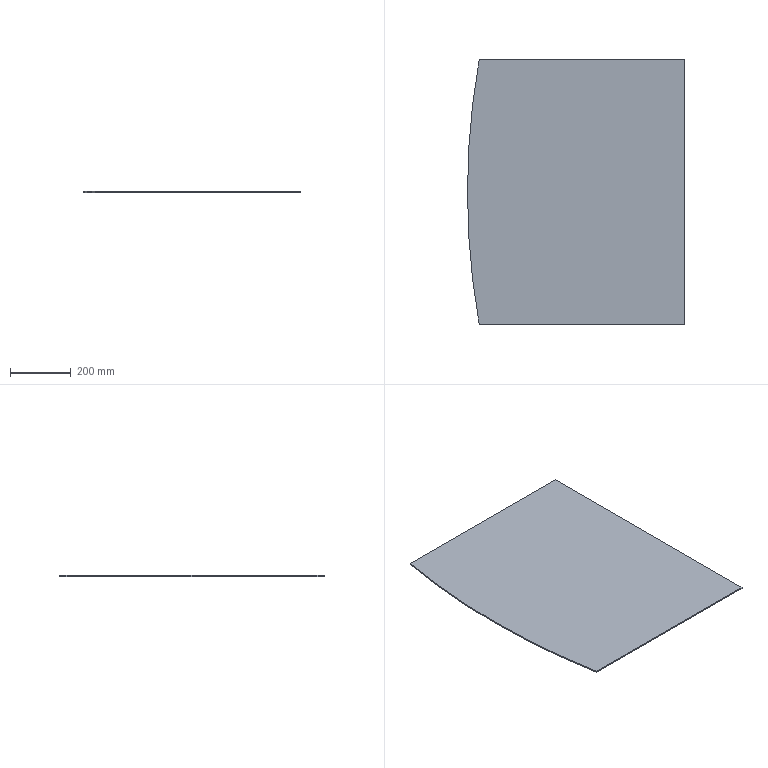Part | STEP file | 09-End cover plate | 1 solid | 7 faces | box 714.448 x 870 x 4 mm | volume 2441819 mm3 | plane 5 | cylinder 2 | commonest cylinder face diameters 4960 x2
STEP:
#1=CARTESIAN_POINT('',(0.,0.,0.));
#2=DIRECTION('',(0.,0.,1.));
#3=DIRECTION('',(1.,0.,0.));
#4=AXIS2_PLACEMENT_3D('',#1,#2,#3);
#5=CARTESIAN_POINT('',(-714.448,-435.,4.));
#6=VERTEX_POINT('',#5);
#7=CARTESIAN_POINT('',(-676.,-870.,4.));
#8=VERTEX_POINT('',#7);
#9=CARTESIAN_POINT('',(1765.552,-435.,4.));
#10=DIRECTION('',(0.,0.,1.));
#11=DIRECTION('',(1.,0.,0.));
#12=AXIS2_PLACEMENT_3D('',#9,#10,#11);
#13=CIRCLE('',#12,2480.);
#14=CARTESIAN_POINT('',(1765.552,-435.,4.));
#15=DIRECTION('',(0.,0.,-1.));
#16=DIRECTION('',(-1.,0.,0.));
#17=AXIS2_PLACEMENT_3D('',#14,#15,#16);
#18=CYLINDRICAL_SURFACE('',#17,2480.);
#19=CARTESIAN_POINT('',(9.425,0.));
#20=DIRECTION('',(-1.,0.));
#21=VECTOR('',#20,1.);
#22=LINE('',#19,#21);
#23=(GEOMETRIC_REPRESENTATION_CONTEXT(2)PARAMETRIC_REPRESENTATION_CONTEXT()REPRESENTATION_CONTEXT('',''));
#24=DEFINITIONAL_REPRESENTATION('',(#22),#23);
#25=PCURVE('',#18,#24);
#26=CARTESIAN_POINT('',(1765.552,-435.,4.));
#27=DIRECTION('',(0.,0.,1.));
#28=DIRECTION('',(1.,0.,0.));
#29=AXIS2_PLACEMENT_3D('',#26,#27,#28);
#30=PLANE('',#29);
#31=CARTESIAN_POINT('',(0.,0.));
#32=DIRECTION('',(1.,0.));
#33=AXIS2_PLACEMENT_2D('',#31,#32);
#34=CIRCLE('',#33,2480.);
#35=(GEOMETRIC_REPRESENTATION_CONTEXT(2)PARAMETRIC_REPRESENTATION_CONTEXT()REPRESENTATION_CONTEXT('',''));
#36=DEFINITIONAL_REPRESENTATION('',(#34),#35);
#37=PCURVE('',#30,#36);
#38=SURFACE_CURVE('',#13,(#25,#37),.PCURVE_S1.);
#39=EDGE_CURVE('',#6,#8,#38,.T.);
#40=ORIENTED_EDGE('',*,*,#39,.F.);
#41=CARTESIAN_POINT('',(-714.448,-435.,0.));
#42=VERTEX_POINT('',#41);
#43=CARTESIAN_POINT('',(-714.448,-435.,4.));
#44=DIRECTION('',(0.,0.,-1.));
#45=VECTOR('',#44,1.);
#46=LINE('',#43,#45);
#47=CARTESIAN_POINT('',(6.283,0.));
#48=DIRECTION('',(0.,1.));
#49=VECTOR('',#48,1.);
#50=LINE('',#47,#49);
#51=(GEOMETRIC_REPRESENTATION_CONTEXT(2)PARAMETRIC_REPRESENTATION_CONTEXT()REPRESENTATION_CONTEXT('',''));
#52=DEFINITIONAL_REPRESENTATION('',(#50),#51);
#53=PCURVE('',#18,#52);
#54=CARTESIAN_POINT('',(1765.552,-435.,4.));
#55=DIRECTION('',(0.,0.,-1.));
#56=DIRECTION('',(-1.,0.,0.));
#57=AXIS2_PLACEMENT_3D('',#54,#55,#56);
#58=CYLINDRICAL_SURFACE('',#57,2480.);
#59=CARTESIAN_POINT('',(0.,0.));
#60=DIRECTION('',(0.,1.));
#61=VECTOR('',#60,1.);
#62=LINE('',#59,#61);
#63=(GEOMETRIC_REPRESENTATION_CONTEXT(2)PARAMETRIC_REPRESENTATION_CONTEXT()REPRESENTATION_CONTEXT('',''));
#64=DEFINITIONAL_REPRESENTATION('',(#62),#63);
#65=PCURVE('',#58,#64);
#66=SURFACE_CURVE('',#46,(#53,#65),.PCURVE_S1.);
#67=EDGE_CURVE('',#6,#42,#66,.T.);
#68=ORIENTED_EDGE('',*,*,#67,.T.);
#69=CARTESIAN_POINT('',(-676.,-870.,0.));
#70=VERTEX_POINT('',#69);
#71=CARTESIAN_POINT('',(1765.552,-435.,0.));
#72=DIRECTION('',(0.,0.,1.));
#73=DIRECTION('',(1.,0.,0.));
#74=AXIS2_PLACEMENT_3D('',#71,#72,#73);
#75=CIRCLE('',#74,2480.);
#76=CARTESIAN_POINT('',(9.425,4.));
#77=DIRECTION('',(-1.,0.));
#78=VECTOR('',#77,1.);
#79=LINE('',#76,#78);
#80=(GEOMETRIC_REPRESENTATION_CONTEXT(2)PARAMETRIC_REPRESENTATION_CONTEXT()REPRESENTATION_CONTEXT('',''));
#81=DEFINITIONAL_REPRESENTATION('',(#79),#80);
#82=PCURVE('',#18,#81);
#83=CARTESIAN_POINT('',(1765.552,-435.,0.));
#84=DIRECTION('',(0.,0.,1.));
#85=DIRECTION('',(1.,0.,0.));
#86=AXIS2_PLACEMENT_3D('',#83,#84,#85);
#87=PLANE('',#86);
#88=CARTESIAN_POINT('',(0.,0.));
#89=DIRECTION('',(1.,0.));
#90=AXIS2_PLACEMENT_2D('',#88,#89);
#91=CIRCLE('',#90,2480.);
#92=(GEOMETRIC_REPRESENTATION_CONTEXT(2)PARAMETRIC_REPRESENTATION_CONTEXT()REPRESENTATION_CONTEXT('',''));
#93=DEFINITIONAL_REPRESENTATION('',(#91),#92);
#94=PCURVE('',#87,#93);
#95=SURFACE_CURVE('',#75,(#82,#94),.PCURVE_S1.);
#96=EDGE_CURVE('',#42,#70,#95,.T.);
#97=ORIENTED_EDGE('',*,*,#96,.T.);
#98=CARTESIAN_POINT('',(-676.,-870.,4.));
#99=DIRECTION('',(0.,0.,-1.));
#100=VECTOR('',#99,1.);
#101=LINE('',#98,#100);
#102=CARTESIAN_POINT('',(6.107,0.));
#103=DIRECTION('',(0.,1.));
#104=VECTOR('',#103,1.);
#105=LINE('',#102,#104);
#106=(GEOMETRIC_REPRESENTATION_CONTEXT(2)PARAMETRIC_REPRESENTATION_CONTEXT()REPRESENTATION_CONTEXT('',''));
#107=DEFINITIONAL_REPRESENTATION('',(#105),#106);
#108=PCURVE('',#18,#107);
#109=CARTESIAN_POINT('',(0.,-870.,4.));
#110=DIRECTION('',(0.,1.,0.));
#111=DIRECTION('',(-1.,0.,0.));
#112=AXIS2_PLACEMENT_3D('',#109,#110,#111);
#113=PLANE('',#112);
#114=CARTESIAN_POINT('',(676.,0.));
#115=DIRECTION('',(0.,-1.));
#116=VECTOR('',#115,1.);
#117=LINE('',#114,#116);
#118=(GEOMETRIC_REPRESENTATION_CONTEXT(2)PARAMETRIC_REPRESENTATION_CONTEXT()REPRESENTATION_CONTEXT('',''));
#119=DEFINITIONAL_REPRESENTATION('',(#117),#118);
#120=PCURVE('',#113,#119);
#121=SURFACE_CURVE('',#101,(#108,#120),.PCURVE_S1.);
#122=EDGE_CURVE('',#8,#70,#121,.T.);
#123=ORIENTED_EDGE('',*,*,#122,.F.);
#124=EDGE_LOOP('',(#40,#68,#97,#123));
#125=FACE_BOUND('',#124,.T.);
#126=ADVANCED_FACE('',(#125),#18,.T.);
#127=CARTESIAN_POINT('',(0.,-870.,0.));
#128=VERTEX_POINT('',#127);
#129=CARTESIAN_POINT('',(0.,0.,0.));
#130=VERTEX_POINT('',#129);
#131=CARTESIAN_POINT('',(0.,0.,0.));
#132=DIRECTION('',(0.,1.,0.));
#133=VECTOR('',#132,1.);
#134=LINE('',#131,#133);
#135=CARTESIAN_POINT('',(0.,0.,4.));
#136=DIRECTION('',(-1.,0.,0.));
#137=DIRECTION('',(0.,-1.,0.));
#138=AXIS2_PLACEMENT_3D('',#135,#136,#137);
#139=PLANE('',#138);
#140=CARTESIAN_POINT('',(0.,-4.));
#141=DIRECTION('',(-1.,0.));
#142=VECTOR('',#141,1.);
#143=LINE('',#140,#142);
#144=(GEOMETRIC_REPRESENTATION_CONTEXT(2)PARAMETRIC_REPRESENTATION_CONTEXT()REPRESENTATION_CONTEXT('',''));
#145=DEFINITIONAL_REPRESENTATION('',(#143),#144);
#146=PCURVE('',#139,#145);
#147=CARTESIAN_POINT('',(-1765.552,435.));
#148=DIRECTION('',(0.,1.));
#149=VECTOR('',#148,1.);
#150=LINE('',#147,#149);
#151=(GEOMETRIC_REPRESENTATION_CONTEXT(2)PARAMETRIC_REPRESENTATION_CONTEXT()REPRESENTATION_CONTEXT('',''));
#152=DEFINITIONAL_REPRESENTATION('',(#150),#151);
#153=PCURVE('',#87,#152);
#154=SURFACE_CURVE('',#134,(#146,#153),.PCURVE_S1.);
#155=EDGE_CURVE('',#128,#130,#154,.T.);
#156=ORIENTED_EDGE('',*,*,#155,.T.);
#157=CARTESIAN_POINT('',(0.,0.,4.));
#158=VERTEX_POINT('',#157);
#159=CARTESIAN_POINT('',(0.,0.,4.));
#160=DIRECTION('',(0.,0.,-1.));
#161=VECTOR('',#160,1.);
#162=LINE('',#159,#161);
#163=CARTESIAN_POINT('',(0.,0.));
#164=DIRECTION('',(0.,-1.));
#165=VECTOR('',#164,1.);
#166=LINE('',#163,#165);
#167=(GEOMETRIC_REPRESENTATION_CONTEXT(2)PARAMETRIC_REPRESENTATION_CONTEXT()REPRESENTATION_CONTEXT('',''));
#168=DEFINITIONAL_REPRESENTATION('',(#166),#167);
#169=PCURVE('',#139,#168);
#170=CARTESIAN_POINT('',(0.,0.,4.));
#171=DIRECTION('',(0.,-1.,0.));
#172=DIRECTION('',(1.,0.,0.));
#173=AXIS2_PLACEMENT_3D('',#170,#171,#172);
#174=PLANE('',#173);
#175=CARTESIAN_POINT('',(0.,0.));
#176=DIRECTION('',(0.,-1.));
#177=VECTOR('',#176,1.);
#178=LINE('',#175,#177);
#179=(GEOMETRIC_REPRESENTATION_CONTEXT(2)PARAMETRIC_REPRESENTATION_CONTEXT()REPRESENTATION_CONTEXT('',''));
#180=DEFINITIONAL_REPRESENTATION('',(#178),#179);
#181=PCURVE('',#174,#180);
#182=SURFACE_CURVE('',#162,(#169,#181),.PCURVE_S1.);
#183=EDGE_CURVE('',#158,#130,#182,.T.);
#184=ORIENTED_EDGE('',*,*,#183,.F.);
#185=CARTESIAN_POINT('',(0.,-870.,4.));
#186=VERTEX_POINT('',#185);
#187=CARTESIAN_POINT('',(0.,0.,4.));
#188=DIRECTION('',(0.,1.,0.));
#189=VECTOR('',#188,1.);
#190=LINE('',#187,#189);
#191=CARTESIAN_POINT('',(0.,0.));
#192=DIRECTION('',(-1.,0.));
#193=VECTOR('',#192,1.);
#194=LINE('',#191,#193);
#195=(GEOMETRIC_REPRESENTATION_CONTEXT(2)PARAMETRIC_REPRESENTATION_CONTEXT()REPRESENTATION_CONTEXT('',''));
#196=DEFINITIONAL_REPRESENTATION('',(#194),#195);
#197=PCURVE('',#139,#196);
#198=CARTESIAN_POINT('',(-1765.552,435.));
#199=DIRECTION('',(0.,1.));
#200=VECTOR('',#199,1.);
#201=LINE('',#198,#200);
#202=(GEOMETRIC_REPRESENTATION_CONTEXT(2)PARAMETRIC_REPRESENTATION_CONTEXT()REPRESENTATION_CONTEXT('',''));
#203=DEFINITIONAL_REPRESENTATION('',(#201),#202);
#204=PCURVE('',#30,#203);
#205=SURFACE_CURVE('',#190,(#197,#204),.PCURVE_S1.);
#206=EDGE_CURVE('',#186,#158,#205,.T.);
#207=ORIENTED_EDGE('',*,*,#206,.F.);
#208=CARTESIAN_POINT('',(0.,-870.,4.));
#209=DIRECTION('',(0.,0.,-1.));
#210=VECTOR('',#209,1.);
#211=LINE('',#208,#210);
#212=CARTESIAN_POINT('',(870.,0.));
#213=DIRECTION('',(0.,-1.));
#214=VECTOR('',#213,1.);
#215=LINE('',#212,#214);
#216=(GEOMETRIC_REPRESENTATION_CONTEXT(2)PARAMETRIC_REPRESENTATION_CONTEXT()REPRESENTATION_CONTEXT('',''));
#217=DEFINITIONAL_REPRESENTATION('',(#215),#216);
#218=PCURVE('',#139,#217);
#219=CARTESIAN_POINT('',(0.,0.));
#220=DIRECTION('',(0.,-1.));
#221=VECTOR('',#220,1.);
#222=LINE('',#219,#221);
#223=(GEOMETRIC_REPRESENTATION_CONTEXT(2)PARAMETRIC_REPRESENTATION_CONTEXT()REPRESENTATION_CONTEXT('',''));
#224=DEFINITIONAL_REPRESENTATION('',(#222),#223);
#225=PCURVE('',#113,#224);
#226=SURFACE_CURVE('',#211,(#218,#225),.PCURVE_S1.);
#227=EDGE_CURVE('',#186,#128,#226,.T.);
#228=ORIENTED_EDGE('',*,*,#227,.T.);
#229=EDGE_LOOP('',(#156,#184,#207,#228));
#230=FACE_BOUND('',#229,.T.);
#231=ADVANCED_FACE('',(#230),#139,.F.);
#232=CARTESIAN_POINT('',(-676.,0.,0.));
#233=VERTEX_POINT('',#232);
#234=CARTESIAN_POINT('',(0.,0.,0.));
#235=DIRECTION('',(-1.,0.,0.));
#236=VECTOR('',#235,1.);
#237=LINE('',#234,#236);
#238=CARTESIAN_POINT('',(0.,-4.));
#239=DIRECTION('',(-1.,0.));
#240=VECTOR('',#239,1.);
#241=LINE('',#238,#240);
#242=(GEOMETRIC_REPRESENTATION_CONTEXT(2)PARAMETRIC_REPRESENTATION_CONTEXT()REPRESENTATION_CONTEXT('',''));
#243=DEFINITIONAL_REPRESENTATION('',(#241),#242);
#244=PCURVE('',#174,#243);
#245=CARTESIAN_POINT('',(-1765.552,435.));
#246=DIRECTION('',(-1.,0.));
#247=VECTOR('',#246,1.);
#248=LINE('',#245,#247);
#249=(GEOMETRIC_REPRESENTATION_CONTEXT(2)PARAMETRIC_REPRESENTATION_CONTEXT()REPRESENTATION_CONTEXT('',''));
#250=DEFINITIONAL_REPRESENTATION('',(#248),#249);
#251=PCURVE('',#87,#250);
#252=SURFACE_CURVE('',#237,(#244,#251),.PCURVE_S1.);
#253=EDGE_CURVE('',#130,#233,#252,.T.);
#254=ORIENTED_EDGE('',*,*,#253,.T.);
#255=CARTESIAN_POINT('',(-676.,0.,4.));
#256=VERTEX_POINT('',#255);
#257=CARTESIAN_POINT('',(-676.,0.,4.));
#258=DIRECTION('',(0.,0.,-1.));
#259=VECTOR('',#258,1.);
#260=LINE('',#257,#259);
#261=CARTESIAN_POINT('',(-676.,0.));
#262=DIRECTION('',(0.,-1.));
#263=VECTOR('',#262,1.);
#264=LINE('',#261,#263);
#265=(GEOMETRIC_REPRESENTATION_CONTEXT(2)PARAMETRIC_REPRESENTATION_CONTEXT()REPRESENTATION_CONTEXT('',''));
#266=DEFINITIONAL_REPRESENTATION('',(#264),#265);
#267=PCURVE('',#174,#266);
#268=CARTESIAN_POINT('',(0.1763,0.));
#269=DIRECTION('',(0.,1.));
#270=VECTOR('',#269,1.);
#271=LINE('',#268,#270);
#272=(GEOMETRIC_REPRESENTATION_CONTEXT(2)PARAMETRIC_REPRESENTATION_CONTEXT()REPRESENTATION_CONTEXT('',''));
#273=DEFINITIONAL_REPRESENTATION('',(#271),#272);
#274=PCURVE('',#58,#273);
#275=SURFACE_CURVE('',#260,(#267,#274),.PCURVE_S1.);
#276=EDGE_CURVE('',#256,#233,#275,.T.);
#277=ORIENTED_EDGE('',*,*,#276,.F.);
#278=CARTESIAN_POINT('',(0.,0.,4.));
#279=DIRECTION('',(-1.,0.,0.));
#280=VECTOR('',#279,1.);
#281=LINE('',#278,#280);
#282=CARTESIAN_POINT('',(0.,0.));
#283=DIRECTION('',(-1.,0.));
#284=VECTOR('',#283,1.);
#285=LINE('',#282,#284);
#286=(GEOMETRIC_REPRESENTATION_CONTEXT(2)PARAMETRIC_REPRESENTATION_CONTEXT()REPRESENTATION_CONTEXT('',''));
#287=DEFINITIONAL_REPRESENTATION('',(#285),#286);
#288=PCURVE('',#174,#287);
#289=CARTESIAN_POINT('',(-1765.552,435.));
#290=DIRECTION('',(-1.,0.));
#291=VECTOR('',#290,1.);
#292=LINE('',#289,#291);
#293=(GEOMETRIC_REPRESENTATION_CONTEXT(2)PARAMETRIC_REPRESENTATION_CONTEXT()REPRESENTATION_CONTEXT('',''));
#294=DEFINITIONAL_REPRESENTATION('',(#292),#293);
#295=PCURVE('',#30,#294);
#296=SURFACE_CURVE('',#281,(#288,#295),.PCURVE_S1.);
#297=EDGE_CURVE('',#158,#256,#296,.T.);
#298=ORIENTED_EDGE('',*,*,#297,.F.);
#299=ORIENTED_EDGE('',*,*,#183,.T.);
#300=EDGE_LOOP('',(#254,#277,#298,#299));
#301=FACE_BOUND('',#300,.T.);
#302=ADVANCED_FACE('',(#301),#174,.F.);
#303=ORIENTED_EDGE('',*,*,#67,.F.);
#304=CARTESIAN_POINT('',(1765.552,-435.,4.));
#305=DIRECTION('',(0.,0.,1.));
#306=DIRECTION('',(1.,0.,0.));
#307=AXIS2_PLACEMENT_3D('',#304,#305,#306);
#308=CIRCLE('',#307,2480.);
#309=CARTESIAN_POINT('',(3.142,0.));
#310=DIRECTION('',(-1.,0.));
#311=VECTOR('',#310,1.);
#312=LINE('',#309,#311);
#313=(GEOMETRIC_REPRESENTATION_CONTEXT(2)PARAMETRIC_REPRESENTATION_CONTEXT()REPRESENTATION_CONTEXT('',''));
#314=DEFINITIONAL_REPRESENTATION('',(#312),#313);
#315=PCURVE('',#58,#314);
#316=CARTESIAN_POINT('',(0.,0.));
#317=DIRECTION('',(1.,0.));
#318=AXIS2_PLACEMENT_2D('',#316,#317);
#319=CIRCLE('',#318,2480.);
#320=(GEOMETRIC_REPRESENTATION_CONTEXT(2)PARAMETRIC_REPRESENTATION_CONTEXT()REPRESENTATION_CONTEXT('',''));
#321=DEFINITIONAL_REPRESENTATION('',(#319),#320);
#322=PCURVE('',#30,#321);
#323=SURFACE_CURVE('',#308,(#315,#322),.PCURVE_S1.);
#324=EDGE_CURVE('',#256,#6,#323,.T.);
#325=ORIENTED_EDGE('',*,*,#324,.F.);
#326=ORIENTED_EDGE('',*,*,#276,.T.);
#327=CARTESIAN_POINT('',(1765.552,-435.,0.));
#328=DIRECTION('',(0.,0.,1.));
#329=DIRECTION('',(1.,0.,0.));
#330=AXIS2_PLACEMENT_3D('',#327,#328,#329);
#331=CIRCLE('',#330,2480.);
#332=CARTESIAN_POINT('',(3.142,4.));
#333=DIRECTION('',(-1.,0.));
#334=VECTOR('',#333,1.);
#335=LINE('',#332,#334);
#336=(GEOMETRIC_REPRESENTATION_CONTEXT(2)PARAMETRIC_REPRESENTATION_CONTEXT()REPRESENTATION_CONTEXT('',''));
#337=DEFINITIONAL_REPRESENTATION('',(#335),#336);
#338=PCURVE('',#58,#337);
#339=CARTESIAN_POINT('',(0.,0.));
#340=DIRECTION('',(1.,0.));
#341=AXIS2_PLACEMENT_2D('',#339,#340);
#342=CIRCLE('',#341,2480.);
#343=(GEOMETRIC_REPRESENTATION_CONTEXT(2)PARAMETRIC_REPRESENTATION_CONTEXT()REPRESENTATION_CONTEXT('',''));
#344=DEFINITIONAL_REPRESENTATION('',(#342),#343);
#345=PCURVE('',#87,#344);
#346=SURFACE_CURVE('',#331,(#338,#345),.PCURVE_S1.);
#347=EDGE_CURVE('',#233,#42,#346,.T.);
#348=ORIENTED_EDGE('',*,*,#347,.T.);
#349=EDGE_LOOP('',(#303,#325,#326,#348));
#350=FACE_BOUND('',#349,.T.);
#351=ADVANCED_FACE('',(#350),#58,.T.);
#352=CARTESIAN_POINT('',(0.,-870.,0.));
#353=DIRECTION('',(1.,0.,0.));
#354=VECTOR('',#353,1.);
#355=LINE('',#352,#354);
#356=CARTESIAN_POINT('',(0.,-4.));
#357=DIRECTION('',(-1.,0.));
#358=VECTOR('',#357,1.);
#359=LINE('',#356,#358);
#360=(GEOMETRIC_REPRESENTATION_CONTEXT(2)PARAMETRIC_REPRESENTATION_CONTEXT()REPRESENTATION_CONTEXT('',''));
#361=DEFINITIONAL_REPRESENTATION('',(#359),#360);
#362=PCURVE('',#113,#361);
#363=CARTESIAN_POINT('',(-1765.552,-435.));
#364=DIRECTION('',(1.,0.));
#365=VECTOR('',#364,1.);
#366=LINE('',#363,#365);
#367=(GEOMETRIC_REPRESENTATION_CONTEXT(2)PARAMETRIC_REPRESENTATION_CONTEXT()REPRESENTATION_CONTEXT('',''));
#368=DEFINITIONAL_REPRESENTATION('',(#366),#367);
#369=PCURVE('',#87,#368);
#370=SURFACE_CURVE('',#355,(#362,#369),.PCURVE_S1.);
#371=EDGE_CURVE('',#70,#128,#370,.T.);
#372=ORIENTED_EDGE('',*,*,#371,.T.);
#373=ORIENTED_EDGE('',*,*,#227,.F.);
#374=CARTESIAN_POINT('',(0.,-870.,4.));
#375=DIRECTION('',(1.,0.,0.));
#376=VECTOR('',#375,1.);
#377=LINE('',#374,#376);
#378=CARTESIAN_POINT('',(0.,0.));
#379=DIRECTION('',(-1.,0.));
#380=VECTOR('',#379,1.);
#381=LINE('',#378,#380);
#382=(GEOMETRIC_REPRESENTATION_CONTEXT(2)PARAMETRIC_REPRESENTATION_CONTEXT()REPRESENTATION_CONTEXT('',''));
#383=DEFINITIONAL_REPRESENTATION('',(#381),#382);
#384=PCURVE('',#113,#383);
#385=CARTESIAN_POINT('',(-1765.552,-435.));
#386=DIRECTION('',(1.,0.));
#387=VECTOR('',#386,1.);
#388=LINE('',#385,#387);
#389=(GEOMETRIC_REPRESENTATION_CONTEXT(2)PARAMETRIC_REPRESENTATION_CONTEXT()REPRESENTATION_CONTEXT('',''));
#390=DEFINITIONAL_REPRESENTATION('',(#388),#389);
#391=PCURVE('',#30,#390);
#392=SURFACE_CURVE('',#377,(#384,#391),.PCURVE_S1.);
#393=EDGE_CURVE('',#8,#186,#392,.T.);
#394=ORIENTED_EDGE('',*,*,#393,.F.);
#395=ORIENTED_EDGE('',*,*,#122,.T.);
#396=EDGE_LOOP('',(#372,#373,#394,#395));
#397=FACE_BOUND('',#396,.T.);
#398=ADVANCED_FACE('',(#397),#113,.F.);
#399=ORIENTED_EDGE('',*,*,#206,.T.);
#400=ORIENTED_EDGE('',*,*,#297,.T.);
#401=ORIENTED_EDGE('',*,*,#324,.T.);
#402=ORIENTED_EDGE('',*,*,#39,.T.);
#403=ORIENTED_EDGE('',*,*,#393,.T.);
#404=EDGE_LOOP('',(#399,#400,#401,#402,#403));
#405=FACE_BOUND('',#404,.T.);
#406=ADVANCED_FACE('',(#405),#30,.T.);
#407=ORIENTED_EDGE('',*,*,#155,.F.);
#408=ORIENTED_EDGE('',*,*,#371,.F.);
#409=ORIENTED_EDGE('',*,*,#96,.F.);
#410=ORIENTED_EDGE('',*,*,#347,.F.);
#411=ORIENTED_EDGE('',*,*,#253,.F.);
#412=EDGE_LOOP('',(#407,#408,#409,#410,#411));
#413=FACE_BOUND('',#412,.T.);
#414=ADVANCED_FACE('',(#413),#87,.F.);
#415=CLOSED_SHELL('',(#126,#231,#302,#351,#398,#406,#414));
#416=MANIFOLD_SOLID_BREP('',#415);
#417=(LENGTH_UNIT()NAMED_UNIT(*)SI_UNIT(.MILLI.,.METRE.));
#418=UNCERTAINTY_MEASURE_WITH_UNIT(LENGTH_MEASURE(0.0000001),#417,'','');
#419=(NAMED_UNIT(*)PLANE_ANGLE_UNIT()SI_UNIT($,.RADIAN.));
#420=(NAMED_UNIT(*)SI_UNIT($,.STERADIAN.)SOLID_ANGLE_UNIT());
#421=(GEOMETRIC_REPRESENTATION_CONTEXT(3)GLOBAL_UNCERTAINTY_ASSIGNED_CONTEXT((#418))GLOBAL_UNIT_ASSIGNED_CONTEXT((#417,#419,#420))REPRESENTATION_CONTEXT('',''));
#422=ADVANCED_BREP_SHAPE_REPRESENTATION('',(#4,#416),#421);